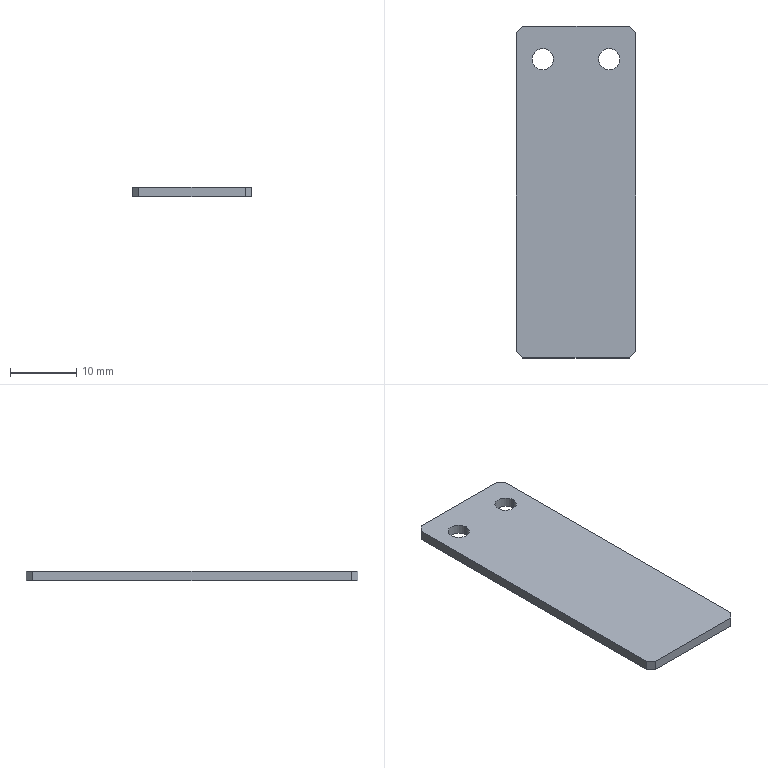Part | SolidWorks | features Chamfer 1, Extrusion 1, HoleWzd 1 | 1 solid | 14 faces | box 18 x 50 x 1.5 mm | volume 1323 mm3 | plane 10 | cylinder 4 | commonest cylinder face diameters 3.2 x4
STEP:
#1=CARTESIAN_POINT('',(-6.6,20.,0.));
#2=VERTEX_POINT('',#1);
#3=CARTESIAN_POINT('',(-3.4,20.,0.));
#4=VERTEX_POINT('',#3);
#5=CARTESIAN_POINT('',(-5.,20.,0.));
#6=DIRECTION('',(0.,0.,1.));
#7=DIRECTION('',(1.,0.,0.));
#8=AXIS2_PLACEMENT_3D('',#5,#6,#7);
#9=CIRCLE('',#8,1.6);
#10=EDGE_CURVE('',#2,#4,#9,.T.);
#11=ORIENTED_EDGE('',*,*,#10,.F.);
#12=CARTESIAN_POINT('',(-6.6,20.,1.5));
#13=VERTEX_POINT('',#12);
#14=CARTESIAN_POINT('',(-6.6,20.,1.5));
#15=DIRECTION('',(0.,0.,1.));
#16=VECTOR('',#15,1000.);
#17=LINE('',#14,#16);
#18=EDGE_CURVE('',#2,#13,#17,.T.);
#19=ORIENTED_EDGE('',*,*,#18,.T.);
#20=CARTESIAN_POINT('',(-3.4,20.,1.5));
#21=VERTEX_POINT('',#20);
#22=CARTESIAN_POINT('',(-5.,20.,1.5));
#23=DIRECTION('',(0.,0.,1.));
#24=DIRECTION('',(1.,0.,0.));
#25=AXIS2_PLACEMENT_3D('',#22,#23,#24);
#26=CIRCLE('',#25,1.6);
#27=EDGE_CURVE('',#13,#21,#26,.T.);
#28=ORIENTED_EDGE('',*,*,#27,.T.);
#29=CARTESIAN_POINT('',(-3.4,20.,1.5));
#30=DIRECTION('',(0.,0.,1.));
#31=VECTOR('',#30,1000.);
#32=LINE('',#29,#31);
#33=EDGE_CURVE('',#4,#21,#32,.T.);
#34=ORIENTED_EDGE('',*,*,#33,.F.);
#35=EDGE_LOOP('',(#11,#19,#28,#34));
#36=FACE_OUTER_BOUND('',#35,.T.);
#37=CARTESIAN_POINT('',(-5.,20.,1.5));
#38=DIRECTION('',(0.,0.,1.));
#39=DIRECTION('',(1.,0.,0.));
#40=AXIS2_PLACEMENT_3D('',#37,#38,#39);
#41=CYLINDRICAL_SURFACE('',#40,1.6);
#42=ADVANCED_FACE('',(#36),#41,.F.);
#43=CARTESIAN_POINT('',(3.4,20.,0.));
#44=VERTEX_POINT('',#43);
#45=CARTESIAN_POINT('',(6.6,20.,0.));
#46=VERTEX_POINT('',#45);
#47=CARTESIAN_POINT('',(5.,20.,0.));
#48=DIRECTION('',(0.,0.,1.));
#49=DIRECTION('',(1.,0.,0.));
#50=AXIS2_PLACEMENT_3D('',#47,#48,#49);
#51=CIRCLE('',#50,1.6);
#52=EDGE_CURVE('',#44,#46,#51,.T.);
#53=ORIENTED_EDGE('',*,*,#52,.F.);
#54=CARTESIAN_POINT('',(3.4,20.,1.5));
#55=VERTEX_POINT('',#54);
#56=CARTESIAN_POINT('',(3.4,20.,1.5));
#57=DIRECTION('',(0.,0.,1.));
#58=VECTOR('',#57,1000.);
#59=LINE('',#56,#58);
#60=EDGE_CURVE('',#44,#55,#59,.T.);
#61=ORIENTED_EDGE('',*,*,#60,.T.);
#62=CARTESIAN_POINT('',(6.6,20.,1.5));
#63=VERTEX_POINT('',#62);
#64=CARTESIAN_POINT('',(5.,20.,1.5));
#65=DIRECTION('',(0.,0.,1.));
#66=DIRECTION('',(1.,0.,0.));
#67=AXIS2_PLACEMENT_3D('',#64,#65,#66);
#68=CIRCLE('',#67,1.6);
#69=EDGE_CURVE('',#55,#63,#68,.T.);
#70=ORIENTED_EDGE('',*,*,#69,.T.);
#71=CARTESIAN_POINT('',(6.6,20.,1.5));
#72=DIRECTION('',(0.,0.,1.));
#73=VECTOR('',#72,1000.);
#74=LINE('',#71,#73);
#75=EDGE_CURVE('',#46,#63,#74,.T.);
#76=ORIENTED_EDGE('',*,*,#75,.F.);
#77=EDGE_LOOP('',(#53,#61,#70,#76));
#78=FACE_OUTER_BOUND('',#77,.T.);
#79=CARTESIAN_POINT('',(5.,20.,1.5));
#80=DIRECTION('',(0.,0.,1.));
#81=DIRECTION('',(1.,0.,0.));
#82=AXIS2_PLACEMENT_3D('',#79,#80,#81);
#83=CYLINDRICAL_SURFACE('',#82,1.6);
#84=ADVANCED_FACE('',(#78),#83,.F.);
#85=CARTESIAN_POINT('',(9.,-24.,0.));
#86=VERTEX_POINT('',#85);
#87=CARTESIAN_POINT('',(9.,24.,0.));
#88=VERTEX_POINT('',#87);
#89=CARTESIAN_POINT('',(9.,25.,0.));
#90=DIRECTION('',(0.,1.,0.));
#91=VECTOR('',#90,1000.);
#92=LINE('',#89,#91);
#93=EDGE_CURVE('',#86,#88,#92,.T.);
#94=ORIENTED_EDGE('',*,*,#93,.T.);
#95=CARTESIAN_POINT('',(9.,24.,1.5));
#96=VERTEX_POINT('',#95);
#97=CARTESIAN_POINT('',(9.,24.,1.5));
#98=DIRECTION('',(0.,0.,1.));
#99=VECTOR('',#98,1000.);
#100=LINE('',#97,#99);
#101=EDGE_CURVE('',#88,#96,#100,.T.);
#102=ORIENTED_EDGE('',*,*,#101,.T.);
#103=CARTESIAN_POINT('',(9.,-24.,1.5));
#104=VERTEX_POINT('',#103);
#105=CARTESIAN_POINT('',(9.,25.,1.5));
#106=DIRECTION('',(0.,1.,0.));
#107=VECTOR('',#106,1000.);
#108=LINE('',#105,#107);
#109=EDGE_CURVE('',#104,#96,#108,.T.);
#110=ORIENTED_EDGE('',*,*,#109,.F.);
#111=CARTESIAN_POINT('',(9.,-24.,1.5));
#112=DIRECTION('',(0.,0.,-1.));
#113=VECTOR('',#112,1000.);
#114=LINE('',#111,#113);
#115=EDGE_CURVE('',#104,#86,#114,.T.);
#116=ORIENTED_EDGE('',*,*,#115,.T.);
#117=EDGE_LOOP('',(#94,#102,#110,#116));
#118=FACE_OUTER_BOUND('',#117,.T.);
#119=CARTESIAN_POINT('',(9.,25.,1.5));
#120=DIRECTION('',(-1.,0.,0.));
#121=DIRECTION('',(0.,-1.,0.));
#122=AXIS2_PLACEMENT_3D('',#119,#120,#121);
#123=PLANE('',#122);
#124=ADVANCED_FACE('',(#118),#123,.F.);
#125=CARTESIAN_POINT('',(8.,25.,0.));
#126=VERTEX_POINT('',#125);
#127=CARTESIAN_POINT('',(-8.,25.,0.));
#128=VERTEX_POINT('',#127);
#129=CARTESIAN_POINT('',(-9.,25.,0.));
#130=DIRECTION('',(-1.,0.,0.));
#131=VECTOR('',#130,1000.);
#132=LINE('',#129,#131);
#133=EDGE_CURVE('',#126,#128,#132,.T.);
#134=ORIENTED_EDGE('',*,*,#133,.T.);
#135=CARTESIAN_POINT('',(-8.,25.,1.5));
#136=VERTEX_POINT('',#135);
#137=CARTESIAN_POINT('',(-8.,25.,1.5));
#138=DIRECTION('',(0.,0.,1.));
#139=VECTOR('',#138,1000.);
#140=LINE('',#137,#139);
#141=EDGE_CURVE('',#128,#136,#140,.T.);
#142=ORIENTED_EDGE('',*,*,#141,.T.);
#143=CARTESIAN_POINT('',(8.,25.,1.5));
#144=VERTEX_POINT('',#143);
#145=CARTESIAN_POINT('',(-9.,25.,1.5));
#146=DIRECTION('',(-1.,0.,0.));
#147=VECTOR('',#146,1000.);
#148=LINE('',#145,#147);
#149=EDGE_CURVE('',#144,#136,#148,.T.);
#150=ORIENTED_EDGE('',*,*,#149,.F.);
#151=CARTESIAN_POINT('',(8.,25.,1.5));
#152=DIRECTION('',(0.,0.,-1.));
#153=VECTOR('',#152,1000.);
#154=LINE('',#151,#153);
#155=EDGE_CURVE('',#144,#126,#154,.T.);
#156=ORIENTED_EDGE('',*,*,#155,.T.);
#157=EDGE_LOOP('',(#134,#142,#150,#156));
#158=FACE_OUTER_BOUND('',#157,.T.);
#159=CARTESIAN_POINT('',(-9.,25.,1.5));
#160=DIRECTION('',(0.,-1.,0.));
#161=DIRECTION('',(0.,0.,-1.));
#162=AXIS2_PLACEMENT_3D('',#159,#160,#161);
#163=PLANE('',#162);
#164=ADVANCED_FACE('',(#158),#163,.F.);
#165=CARTESIAN_POINT('',(-9.,24.,1.5));
#166=VERTEX_POINT('',#165);
#167=CARTESIAN_POINT('',(-9.,-24.,1.5));
#168=VERTEX_POINT('',#167);
#169=CARTESIAN_POINT('',(-9.,25.,1.5));
#170=DIRECTION('',(0.,-1.,0.));
#171=VECTOR('',#170,1000.);
#172=LINE('',#169,#171);
#173=EDGE_CURVE('',#166,#168,#172,.T.);
#174=ORIENTED_EDGE('',*,*,#173,.F.);
#175=CARTESIAN_POINT('',(-9.,24.,0.));
#176=VERTEX_POINT('',#175);
#177=CARTESIAN_POINT('',(-9.,24.,1.5));
#178=DIRECTION('',(0.,0.,-1.));
#179=VECTOR('',#178,1000.);
#180=LINE('',#177,#179);
#181=EDGE_CURVE('',#166,#176,#180,.T.);
#182=ORIENTED_EDGE('',*,*,#181,.T.);
#183=CARTESIAN_POINT('',(-9.,-24.,0.));
#184=VERTEX_POINT('',#183);
#185=CARTESIAN_POINT('',(-9.,25.,0.));
#186=DIRECTION('',(0.,-1.,0.));
#187=VECTOR('',#186,1000.);
#188=LINE('',#185,#187);
#189=EDGE_CURVE('',#176,#184,#188,.T.);
#190=ORIENTED_EDGE('',*,*,#189,.T.);
#191=CARTESIAN_POINT('',(-9.,-24.,1.5));
#192=DIRECTION('',(0.,0.,1.));
#193=VECTOR('',#192,1000.);
#194=LINE('',#191,#193);
#195=EDGE_CURVE('',#184,#168,#194,.T.);
#196=ORIENTED_EDGE('',*,*,#195,.T.);
#197=EDGE_LOOP('',(#174,#182,#190,#196));
#198=FACE_OUTER_BOUND('',#197,.T.);
#199=CARTESIAN_POINT('',(-9.,25.,1.5));
#200=DIRECTION('',(1.,0.,0.));
#201=DIRECTION('',(0.,1.,0.));
#202=AXIS2_PLACEMENT_3D('',#199,#200,#201);
#203=PLANE('',#202);
#204=ADVANCED_FACE('',(#198),#203,.F.);
#205=CARTESIAN_POINT('',(-8.,-25.,0.));
#206=VERTEX_POINT('',#205);
#207=CARTESIAN_POINT('',(8.,-25.,0.));
#208=VERTEX_POINT('',#207);
#209=CARTESIAN_POINT('',(-9.,-25.,0.));
#210=DIRECTION('',(1.,0.,0.));
#211=VECTOR('',#210,1000.);
#212=LINE('',#209,#211);
#213=EDGE_CURVE('',#206,#208,#212,.T.);
#214=ORIENTED_EDGE('',*,*,#213,.T.);
#215=CARTESIAN_POINT('',(8.,-25.,1.5));
#216=VERTEX_POINT('',#215);
#217=CARTESIAN_POINT('',(8.,-25.,1.5));
#218=DIRECTION('',(0.,0.,1.));
#219=VECTOR('',#218,1000.);
#220=LINE('',#217,#219);
#221=EDGE_CURVE('',#208,#216,#220,.T.);
#222=ORIENTED_EDGE('',*,*,#221,.T.);
#223=CARTESIAN_POINT('',(-8.,-25.,1.5));
#224=VERTEX_POINT('',#223);
#225=CARTESIAN_POINT('',(-9.,-25.,1.5));
#226=DIRECTION('',(1.,0.,0.));
#227=VECTOR('',#226,1000.);
#228=LINE('',#225,#227);
#229=EDGE_CURVE('',#224,#216,#228,.T.);
#230=ORIENTED_EDGE('',*,*,#229,.F.);
#231=CARTESIAN_POINT('',(-8.,-25.,1.5));
#232=DIRECTION('',(0.,0.,-1.));
#233=VECTOR('',#232,1000.);
#234=LINE('',#231,#233);
#235=EDGE_CURVE('',#224,#206,#234,.T.);
#236=ORIENTED_EDGE('',*,*,#235,.T.);
#237=EDGE_LOOP('',(#214,#222,#230,#236));
#238=FACE_OUTER_BOUND('',#237,.T.);
#239=CARTESIAN_POINT('',(-9.,-25.,1.5));
#240=DIRECTION('',(0.,1.,0.));
#241=DIRECTION('',(0.,0.,1.));
#242=AXIS2_PLACEMENT_3D('',#239,#240,#241);
#243=PLANE('',#242);
#244=ADVANCED_FACE('',(#238),#243,.F.);
#245=CARTESIAN_POINT('',(-5.,20.,1.5));
#246=DIRECTION('',(0.,0.,1.));
#247=DIRECTION('',(1.,0.,0.));
#248=AXIS2_PLACEMENT_3D('',#245,#246,#247);
#249=CIRCLE('',#248,1.6);
#250=EDGE_CURVE('',#21,#13,#249,.T.);
#251=ORIENTED_EDGE('',*,*,#250,.F.);
#252=ORIENTED_EDGE('',*,*,#27,.F.);
#253=EDGE_LOOP('',(#251,#252));
#254=FACE_BOUND('',#253,.T.);
#255=CARTESIAN_POINT('',(5.,20.,1.5));
#256=DIRECTION('',(0.,0.,1.));
#257=DIRECTION('',(1.,0.,0.));
#258=AXIS2_PLACEMENT_3D('',#255,#256,#257);
#259=CIRCLE('',#258,1.6);
#260=EDGE_CURVE('',#63,#55,#259,.T.);
#261=ORIENTED_EDGE('',*,*,#260,.F.);
#262=ORIENTED_EDGE('',*,*,#69,.F.);
#263=EDGE_LOOP('',(#261,#262));
#264=FACE_BOUND('',#263,.T.);
#265=ORIENTED_EDGE('',*,*,#149,.T.);
#266=CARTESIAN_POINT('',(-24.5,8.5,1.5));
#267=DIRECTION('',(-0.7071,-0.7071,0.));
#268=VECTOR('',#267,1000.);
#269=LINE('',#266,#268);
#270=EDGE_CURVE('',#136,#166,#269,.T.);
#271=ORIENTED_EDGE('',*,*,#270,.T.);
#272=ORIENTED_EDGE('',*,*,#173,.T.);
#273=CARTESIAN_POINT('',(0.5,-33.5,1.5));
#274=DIRECTION('',(0.7071,-0.7071,0.));
#275=VECTOR('',#274,1000.);
#276=LINE('',#273,#275);
#277=EDGE_CURVE('',#168,#224,#276,.T.);
#278=ORIENTED_EDGE('',*,*,#277,.T.);
#279=ORIENTED_EDGE('',*,*,#229,.T.);
#280=CARTESIAN_POINT('',(8.5,-24.5,1.5));
#281=DIRECTION('',(0.7071,0.7071,0.));
#282=VECTOR('',#281,1000.);
#283=LINE('',#280,#282);
#284=EDGE_CURVE('',#216,#104,#283,.T.);
#285=ORIENTED_EDGE('',*,*,#284,.T.);
#286=ORIENTED_EDGE('',*,*,#109,.T.);
#287=CARTESIAN_POINT('',(33.5,-0.5,1.5));
#288=DIRECTION('',(-0.7071,0.7071,0.));
#289=VECTOR('',#288,1000.);
#290=LINE('',#287,#289);
#291=EDGE_CURVE('',#96,#144,#290,.T.);
#292=ORIENTED_EDGE('',*,*,#291,.T.);
#293=EDGE_LOOP('',(#265,#271,#272,#278,#279,#285,#286,#292));
#294=FACE_OUTER_BOUND('',#293,.T.);
#295=CARTESIAN_POINT('',(9.,-25.,1.5));
#296=DIRECTION('',(0.,0.,1.));
#297=DIRECTION('',(1.,0.,0.));
#298=AXIS2_PLACEMENT_3D('',#295,#296,#297);
#299=PLANE('',#298);
#300=ADVANCED_FACE('',(#254,#264,#294),#299,.T.);
#301=CARTESIAN_POINT('',(-5.,20.,0.));
#302=DIRECTION('',(0.,0.,1.));
#303=DIRECTION('',(1.,0.,0.));
#304=AXIS2_PLACEMENT_3D('',#301,#302,#303);
#305=CIRCLE('',#304,1.6);
#306=EDGE_CURVE('',#4,#2,#305,.T.);
#307=ORIENTED_EDGE('',*,*,#306,.T.);
#308=ORIENTED_EDGE('',*,*,#10,.T.);
#309=EDGE_LOOP('',(#307,#308));
#310=FACE_BOUND('',#309,.T.);
#311=CARTESIAN_POINT('',(5.,20.,0.));
#312=DIRECTION('',(0.,0.,1.));
#313=DIRECTION('',(1.,0.,0.));
#314=AXIS2_PLACEMENT_3D('',#311,#312,#313);
#315=CIRCLE('',#314,1.6);
#316=EDGE_CURVE('',#46,#44,#315,.T.);
#317=ORIENTED_EDGE('',*,*,#316,.T.);
#318=ORIENTED_EDGE('',*,*,#52,.T.);
#319=EDGE_LOOP('',(#317,#318));
#320=FACE_BOUND('',#319,.T.);
#321=ORIENTED_EDGE('',*,*,#189,.F.);
#322=CARTESIAN_POINT('',(-9.,24.,0.));
#323=DIRECTION('',(0.7071,0.7071,0.));
#324=VECTOR('',#323,1000.);
#325=LINE('',#322,#324);
#326=EDGE_CURVE('',#176,#128,#325,.T.);
#327=ORIENTED_EDGE('',*,*,#326,.T.);
#328=ORIENTED_EDGE('',*,*,#133,.F.);
#329=CARTESIAN_POINT('',(8.,25.,0.));
#330=DIRECTION('',(0.7071,-0.7071,0.));
#331=VECTOR('',#330,1000.);
#332=LINE('',#329,#331);
#333=EDGE_CURVE('',#126,#88,#332,.T.);
#334=ORIENTED_EDGE('',*,*,#333,.T.);
#335=ORIENTED_EDGE('',*,*,#93,.F.);
#336=CARTESIAN_POINT('',(9.,-24.,0.));
#337=DIRECTION('',(-0.7071,-0.7071,0.));
#338=VECTOR('',#337,1000.);
#339=LINE('',#336,#338);
#340=EDGE_CURVE('',#86,#208,#339,.T.);
#341=ORIENTED_EDGE('',*,*,#340,.T.);
#342=ORIENTED_EDGE('',*,*,#213,.F.);
#343=CARTESIAN_POINT('',(-8.,-25.,0.));
#344=DIRECTION('',(-0.7071,0.7071,0.));
#345=VECTOR('',#344,1000.);
#346=LINE('',#343,#345);
#347=EDGE_CURVE('',#206,#184,#346,.T.);
#348=ORIENTED_EDGE('',*,*,#347,.T.);
#349=EDGE_LOOP('',(#321,#327,#328,#334,#335,#341,#342,#348));
#350=FACE_OUTER_BOUND('',#349,.T.);
#351=CARTESIAN_POINT('',(9.,-25.,0.));
#352=DIRECTION('',(0.,0.,1.));
#353=DIRECTION('',(1.,0.,0.));
#354=AXIS2_PLACEMENT_3D('',#351,#352,#353);
#355=PLANE('',#354);
#356=ADVANCED_FACE('',(#310,#320,#350),#355,.F.);
#357=ORIENTED_EDGE('',*,*,#60,.F.);
#358=ORIENTED_EDGE('',*,*,#316,.F.);
#359=ORIENTED_EDGE('',*,*,#75,.T.);
#360=ORIENTED_EDGE('',*,*,#260,.T.);
#361=EDGE_LOOP('',(#357,#358,#359,#360));
#362=FACE_OUTER_BOUND('',#361,.T.);
#363=CARTESIAN_POINT('',(5.,20.,1.5));
#364=DIRECTION('',(0.,0.,1.));
#365=DIRECTION('',(1.,0.,0.));
#366=AXIS2_PLACEMENT_3D('',#363,#364,#365);
#367=CYLINDRICAL_SURFACE('',#366,1.6);
#368=ADVANCED_FACE('',(#362),#367,.F.);
#369=ORIENTED_EDGE('',*,*,#18,.F.);
#370=ORIENTED_EDGE('',*,*,#306,.F.);
#371=ORIENTED_EDGE('',*,*,#33,.T.);
#372=ORIENTED_EDGE('',*,*,#250,.T.);
#373=EDGE_LOOP('',(#369,#370,#371,#372));
#374=FACE_OUTER_BOUND('',#373,.T.);
#375=CARTESIAN_POINT('',(-5.,20.,1.5));
#376=DIRECTION('',(0.,0.,1.));
#377=DIRECTION('',(1.,0.,0.));
#378=AXIS2_PLACEMENT_3D('',#375,#376,#377);
#379=CYLINDRICAL_SURFACE('',#378,1.6);
#380=ADVANCED_FACE('',(#374),#379,.F.);
#381=ORIENTED_EDGE('',*,*,#270,.F.);
#382=ORIENTED_EDGE('',*,*,#141,.F.);
#383=ORIENTED_EDGE('',*,*,#326,.F.);
#384=ORIENTED_EDGE('',*,*,#181,.F.);
#385=EDGE_LOOP('',(#381,#382,#383,#384));
#386=FACE_OUTER_BOUND('',#385,.T.);
#387=CARTESIAN_POINT('',(-9.,24.,1.5));
#388=DIRECTION('',(0.7071,-0.7071,0.));
#389=DIRECTION('',(0.7071,0.7071,0.));
#390=AXIS2_PLACEMENT_3D('',#387,#388,#389);
#391=PLANE('',#390);
#392=ADVANCED_FACE('',(#386),#391,.F.);
#393=ORIENTED_EDGE('',*,*,#291,.F.);
#394=ORIENTED_EDGE('',*,*,#101,.F.);
#395=ORIENTED_EDGE('',*,*,#333,.F.);
#396=ORIENTED_EDGE('',*,*,#155,.F.);
#397=EDGE_LOOP('',(#393,#394,#395,#396));
#398=FACE_OUTER_BOUND('',#397,.T.);
#399=CARTESIAN_POINT('',(8.,25.,1.5));
#400=DIRECTION('',(-0.7071,-0.7071,0.));
#401=DIRECTION('',(0.7071,-0.7071,0.));
#402=AXIS2_PLACEMENT_3D('',#399,#400,#401);
#403=PLANE('',#402);
#404=ADVANCED_FACE('',(#398),#403,.F.);
#405=ORIENTED_EDGE('',*,*,#284,.F.);
#406=ORIENTED_EDGE('',*,*,#221,.F.);
#407=ORIENTED_EDGE('',*,*,#340,.F.);
#408=ORIENTED_EDGE('',*,*,#115,.F.);
#409=EDGE_LOOP('',(#405,#406,#407,#408));
#410=FACE_OUTER_BOUND('',#409,.T.);
#411=CARTESIAN_POINT('',(9.,-24.,1.5));
#412=DIRECTION('',(-0.7071,0.7071,0.));
#413=DIRECTION('',(-0.7071,-0.7071,0.));
#414=AXIS2_PLACEMENT_3D('',#411,#412,#413);
#415=PLANE('',#414);
#416=ADVANCED_FACE('',(#410),#415,.F.);
#417=ORIENTED_EDGE('',*,*,#277,.F.);
#418=ORIENTED_EDGE('',*,*,#195,.F.);
#419=ORIENTED_EDGE('',*,*,#347,.F.);
#420=ORIENTED_EDGE('',*,*,#235,.F.);
#421=EDGE_LOOP('',(#417,#418,#419,#420));
#422=FACE_OUTER_BOUND('',#421,.T.);
#423=CARTESIAN_POINT('',(-8.,-25.,1.5));
#424=DIRECTION('',(0.7071,0.7071,0.));
#425=DIRECTION('',(-0.7071,0.7071,0.));
#426=AXIS2_PLACEMENT_3D('',#423,#424,#425);
#427=PLANE('',#426);
#428=ADVANCED_FACE('',(#422),#427,.F.);
#429=CLOSED_SHELL('',(#42,#84,#124,#164,#204,#244,#300,#356,#368,#380,#392,#404,#416,#428));
#430=MANIFOLD_SOLID_BREP('',#429);
#431=CARTESIAN_POINT('',(0.,0.,0.));
#432=DIRECTION('',(0.,0.,1.));
#433=DIRECTION('',(1.,0.,0.));
#434=AXIS2_PLACEMENT_3D('',#431,#432,#433);
#435=(LENGTH_UNIT()NAMED_UNIT(*)SI_UNIT(.MILLI.,.METRE.));
#436=UNCERTAINTY_MEASURE_WITH_UNIT(LENGTH_MEASURE(0.00001),#435,'','');
#437=(NAMED_UNIT(*)PLANE_ANGLE_UNIT()SI_UNIT($,.RADIAN.));
#438=(NAMED_UNIT(*)SI_UNIT($,.STERADIAN.)SOLID_ANGLE_UNIT());
#439=(GEOMETRIC_REPRESENTATION_CONTEXT(3)GLOBAL_UNCERTAINTY_ASSIGNED_CONTEXT((#436))GLOBAL_UNIT_ASSIGNED_CONTEXT((#435,#437,#438))REPRESENTATION_CONTEXT('',''));
#440=ADVANCED_BREP_SHAPE_REPRESENTATION('',(#430,#434),#439);